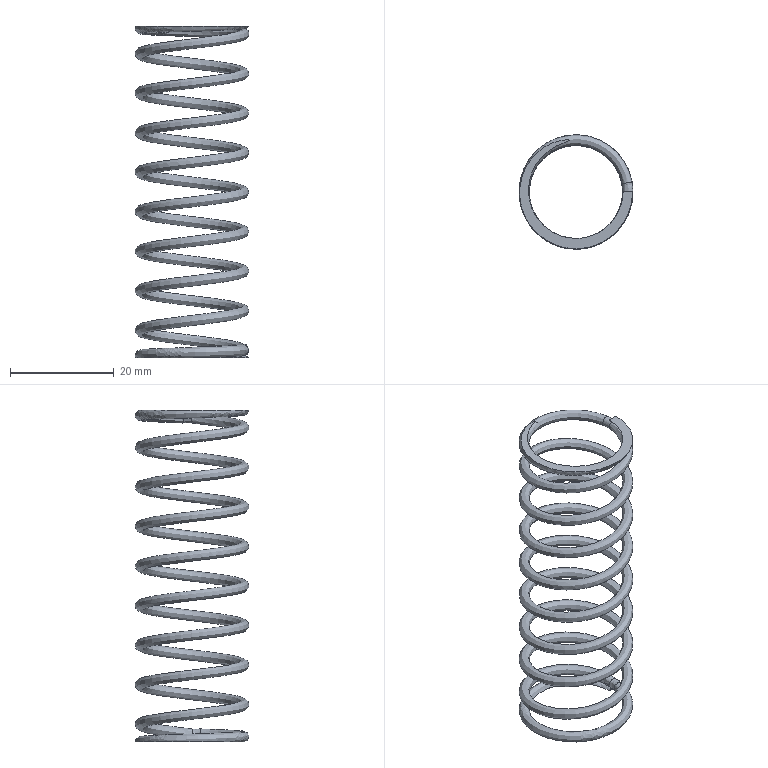Part | NX | features SPLINE_LAW 3, BRIDGE_CURVE 2, DATUM_CSYS 2, DATUM_PLANE 2, TRIM BODY 2, ABSOLUTE_DATUM_AXIS 1, ABSOLUTE_DATUM_PLANE 1, DATUM_ON_PATH 1, FLEXIBLE_PART 1, FSET 1, SKETCH 1, SKIN 1 | 1 solid | 9 faces | volume 1950 mm3 | spline 5 | plane 4